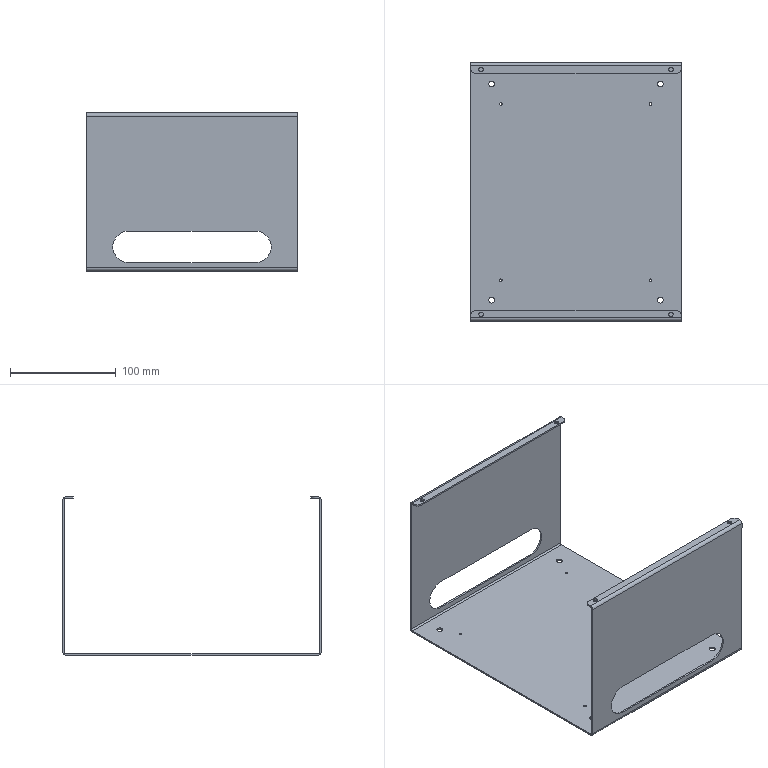Part | NX | features BREP 1 | 1 solid | 46 faces | box 200 x 245 x 150 mm | volume 153333 mm3 | cylinder 28 | plane 18 | commonest cylinder face diameters 2.5 x4 3 x4 4.2 x4 5.5 x4 6 x4 10 x4
STEP:
#1=CARTESIAN_POINT('',(-69.998,-83.5,0.));
#2=VERTEX_POINT('',#1);
#3=CARTESIAN_POINT('',(-71.248,-83.5,0.));
#4=DIRECTION('',(0.,0.,1.));
#5=DIRECTION('',(1.,0.,0.));
#6=AXIS2_PLACEMENT_3D('',#3,#4,#5);
#7=CIRCLE('',#6,1.25);
#8=EDGE_CURVE('',#2,#2,#7,.T.);
#9=ORIENTED_EDGE('',*,*,#8,.T.);
#10=EDGE_LOOP('',(#9));
#11=FACE_BOUND('',#10,.T.);
#12=CARTESIAN_POINT('',(-69.998,-83.5,-1.5));
#13=VERTEX_POINT('',#12);
#14=CARTESIAN_POINT('',(-71.248,-83.5,-1.5));
#15=DIRECTION('',(0.,0.,1.));
#16=DIRECTION('',(1.,0.,0.));
#17=AXIS2_PLACEMENT_3D('',#14,#15,#16);
#18=CIRCLE('',#17,1.25);
#19=EDGE_CURVE('',#13,#13,#18,.T.);
#20=ORIENTED_EDGE('',*,*,#19,.F.);
#21=EDGE_LOOP('',(#20));
#22=FACE_BOUND('',#21,.T.);
#23=CARTESIAN_POINT('',(-71.248,-83.5,0.));
#24=DIRECTION('',(0.,0.,1.));
#25=DIRECTION('',(1.,0.,0.));
#26=AXIS2_PLACEMENT_3D('',#23,#24,#25);
#27=CYLINDRICAL_SURFACE('',#26,1.25);
#28=ADVANCED_FACE('',(#11,#22),#27,.F.);
#29=CARTESIAN_POINT('',(72.002,-83.5,0.));
#30=VERTEX_POINT('',#29);
#31=CARTESIAN_POINT('',(70.752,-83.5,0.));
#32=DIRECTION('',(0.,0.,1.));
#33=DIRECTION('',(1.,0.,0.));
#34=AXIS2_PLACEMENT_3D('',#31,#32,#33);
#35=CIRCLE('',#34,1.25);
#36=EDGE_CURVE('',#30,#30,#35,.T.);
#37=ORIENTED_EDGE('',*,*,#36,.T.);
#38=EDGE_LOOP('',(#37));
#39=FACE_BOUND('',#38,.T.);
#40=CARTESIAN_POINT('',(72.002,-83.5,-1.5));
#41=VERTEX_POINT('',#40);
#42=CARTESIAN_POINT('',(70.752,-83.5,-1.5));
#43=DIRECTION('',(0.,0.,1.));
#44=DIRECTION('',(1.,0.,0.));
#45=AXIS2_PLACEMENT_3D('',#42,#43,#44);
#46=CIRCLE('',#45,1.25);
#47=EDGE_CURVE('',#41,#41,#46,.T.);
#48=ORIENTED_EDGE('',*,*,#47,.F.);
#49=EDGE_LOOP('',(#48));
#50=FACE_BOUND('',#49,.T.);
#51=CARTESIAN_POINT('',(70.752,-83.5,0.));
#52=DIRECTION('',(0.,0.,1.));
#53=DIRECTION('',(1.,0.,0.));
#54=AXIS2_PLACEMENT_3D('',#51,#52,#53);
#55=CYLINDRICAL_SURFACE('',#54,1.25);
#56=ADVANCED_FACE('',(#39,#50),#55,.F.);
#57=CARTESIAN_POINT('',(72.002,83.5,0.));
#58=VERTEX_POINT('',#57);
#59=CARTESIAN_POINT('',(70.752,83.5,0.));
#60=DIRECTION('',(0.,0.,1.));
#61=DIRECTION('',(1.,0.,0.));
#62=AXIS2_PLACEMENT_3D('',#59,#60,#61);
#63=CIRCLE('',#62,1.25);
#64=EDGE_CURVE('',#58,#58,#63,.T.);
#65=ORIENTED_EDGE('',*,*,#64,.T.);
#66=EDGE_LOOP('',(#65));
#67=FACE_BOUND('',#66,.T.);
#68=CARTESIAN_POINT('',(72.002,83.5,-1.5));
#69=VERTEX_POINT('',#68);
#70=CARTESIAN_POINT('',(70.752,83.5,-1.5));
#71=DIRECTION('',(0.,0.,1.));
#72=DIRECTION('',(1.,0.,0.));
#73=AXIS2_PLACEMENT_3D('',#70,#71,#72);
#74=CIRCLE('',#73,1.25);
#75=EDGE_CURVE('',#69,#69,#74,.T.);
#76=ORIENTED_EDGE('',*,*,#75,.F.);
#77=EDGE_LOOP('',(#76));
#78=FACE_BOUND('',#77,.T.);
#79=CARTESIAN_POINT('',(70.752,83.5,0.));
#80=DIRECTION('',(0.,0.,1.));
#81=DIRECTION('',(1.,0.,0.));
#82=AXIS2_PLACEMENT_3D('',#79,#80,#81);
#83=CYLINDRICAL_SURFACE('',#82,1.25);
#84=ADVANCED_FACE('',(#67,#78),#83,.F.);
#85=CARTESIAN_POINT('',(-69.998,83.5,0.));
#86=VERTEX_POINT('',#85);
#87=CARTESIAN_POINT('',(-71.248,83.5,0.));
#88=DIRECTION('',(0.,0.,1.));
#89=DIRECTION('',(1.,0.,0.));
#90=AXIS2_PLACEMENT_3D('',#87,#88,#89);
#91=CIRCLE('',#90,1.25);
#92=EDGE_CURVE('',#86,#86,#91,.T.);
#93=ORIENTED_EDGE('',*,*,#92,.T.);
#94=EDGE_LOOP('',(#93));
#95=FACE_BOUND('',#94,.T.);
#96=CARTESIAN_POINT('',(-69.998,83.5,-1.5));
#97=VERTEX_POINT('',#96);
#98=CARTESIAN_POINT('',(-71.248,83.5,-1.5));
#99=DIRECTION('',(0.,0.,1.));
#100=DIRECTION('',(1.,0.,0.));
#101=AXIS2_PLACEMENT_3D('',#98,#99,#100);
#102=CIRCLE('',#101,1.25);
#103=EDGE_CURVE('',#97,#97,#102,.T.);
#104=ORIENTED_EDGE('',*,*,#103,.F.);
#105=EDGE_LOOP('',(#104));
#106=FACE_BOUND('',#105,.T.);
#107=CARTESIAN_POINT('',(-71.248,83.5,0.));
#108=DIRECTION('',(0.,0.,1.));
#109=DIRECTION('',(1.,0.,0.));
#110=AXIS2_PLACEMENT_3D('',#107,#108,#109);
#111=CYLINDRICAL_SURFACE('',#110,1.25);
#112=ADVANCED_FACE('',(#95,#106),#111,.F.);
#113=CARTESIAN_POINT('',(92.1,116.,148.5));
#114=VERTEX_POINT('',#113);
#115=CARTESIAN_POINT('',(90.,116.,148.5));
#116=DIRECTION('',(0.,0.,1.));
#117=DIRECTION('',(1.,0.,0.));
#118=AXIS2_PLACEMENT_3D('',#115,#116,#117);
#119=CIRCLE('',#118,2.1);
#120=EDGE_CURVE('',#114,#114,#119,.T.);
#121=ORIENTED_EDGE('',*,*,#120,.T.);
#122=EDGE_LOOP('',(#121));
#123=FACE_BOUND('',#122,.T.);
#124=CARTESIAN_POINT('',(90.,113.9,147.));
#125=VERTEX_POINT('',#124);
#126=CARTESIAN_POINT('',(90.,116.,147.));
#127=DIRECTION('',(0.,0.,1.));
#128=DIRECTION('',(0.,-1.,0.));
#129=AXIS2_PLACEMENT_3D('',#126,#127,#128);
#130=CIRCLE('',#129,2.1);
#131=EDGE_CURVE('',#125,#125,#130,.T.);
#132=ORIENTED_EDGE('',*,*,#131,.F.);
#133=EDGE_LOOP('',(#132));
#134=FACE_BOUND('',#133,.T.);
#135=CARTESIAN_POINT('',(90.,116.,148.5));
#136=DIRECTION('',(0.,0.,1.));
#137=DIRECTION('',(1.,0.,0.));
#138=AXIS2_PLACEMENT_3D('',#135,#136,#137);
#139=CYLINDRICAL_SURFACE('',#138,2.1);
#140=ADVANCED_FACE('',(#123,#134),#139,.F.);
#141=CARTESIAN_POINT('',(-87.9,116.,148.5));
#142=VERTEX_POINT('',#141);
#143=CARTESIAN_POINT('',(-90.,116.,148.5));
#144=DIRECTION('',(0.,0.,1.));
#145=DIRECTION('',(1.,0.,0.));
#146=AXIS2_PLACEMENT_3D('',#143,#144,#145);
#147=CIRCLE('',#146,2.1);
#148=EDGE_CURVE('',#142,#142,#147,.T.);
#149=ORIENTED_EDGE('',*,*,#148,.T.);
#150=EDGE_LOOP('',(#149));
#151=FACE_BOUND('',#150,.T.);
#152=CARTESIAN_POINT('',(-90.,113.9,147.));
#153=VERTEX_POINT('',#152);
#154=CARTESIAN_POINT('',(-90.,116.,147.));
#155=DIRECTION('',(0.,0.,1.));
#156=DIRECTION('',(0.,-1.,0.));
#157=AXIS2_PLACEMENT_3D('',#154,#155,#156);
#158=CIRCLE('',#157,2.1);
#159=EDGE_CURVE('',#153,#153,#158,.T.);
#160=ORIENTED_EDGE('',*,*,#159,.F.);
#161=EDGE_LOOP('',(#160));
#162=FACE_BOUND('',#161,.T.);
#163=CARTESIAN_POINT('',(-90.,116.,148.5));
#164=DIRECTION('',(0.,0.,1.));
#165=DIRECTION('',(1.,0.,0.));
#166=AXIS2_PLACEMENT_3D('',#163,#164,#165);
#167=CYLINDRICAL_SURFACE('',#166,2.1);
#168=ADVANCED_FACE('',(#151,#162),#167,.F.);
#169=CARTESIAN_POINT('',(-87.9,-116.,148.5));
#170=VERTEX_POINT('',#169);
#171=CARTESIAN_POINT('',(-90.,-116.,148.5));
#172=DIRECTION('',(0.,0.,1.));
#173=DIRECTION('',(1.,0.,0.));
#174=AXIS2_PLACEMENT_3D('',#171,#172,#173);
#175=CIRCLE('',#174,2.1);
#176=EDGE_CURVE('',#170,#170,#175,.T.);
#177=ORIENTED_EDGE('',*,*,#176,.T.);
#178=EDGE_LOOP('',(#177));
#179=FACE_BOUND('',#178,.T.);
#180=CARTESIAN_POINT('',(-90.,-113.9,147.));
#181=VERTEX_POINT('',#180);
#182=CARTESIAN_POINT('',(-90.,-116.,147.));
#183=DIRECTION('',(0.,0.,-1.));
#184=DIRECTION('',(0.,1.,0.));
#185=AXIS2_PLACEMENT_3D('',#182,#183,#184);
#186=CIRCLE('',#185,2.1);
#187=EDGE_CURVE('',#181,#181,#186,.T.);
#188=ORIENTED_EDGE('',*,*,#187,.T.);
#189=EDGE_LOOP('',(#188));
#190=FACE_BOUND('',#189,.T.);
#191=CARTESIAN_POINT('',(-90.,-116.,148.5));
#192=DIRECTION('',(0.,0.,1.));
#193=DIRECTION('',(1.,0.,0.));
#194=AXIS2_PLACEMENT_3D('',#191,#192,#193);
#195=CYLINDRICAL_SURFACE('',#194,2.1);
#196=ADVANCED_FACE('',(#179,#190),#195,.F.);
#197=CARTESIAN_POINT('',(92.1,-116.,148.5));
#198=VERTEX_POINT('',#197);
#199=CARTESIAN_POINT('',(90.,-116.,148.5));
#200=DIRECTION('',(0.,0.,1.));
#201=DIRECTION('',(1.,0.,0.));
#202=AXIS2_PLACEMENT_3D('',#199,#200,#201);
#203=CIRCLE('',#202,2.1);
#204=EDGE_CURVE('',#198,#198,#203,.T.);
#205=ORIENTED_EDGE('',*,*,#204,.T.);
#206=EDGE_LOOP('',(#205));
#207=FACE_BOUND('',#206,.T.);
#208=CARTESIAN_POINT('',(90.,-113.9,147.));
#209=VERTEX_POINT('',#208);
#210=CARTESIAN_POINT('',(90.,-116.,147.));
#211=DIRECTION('',(0.,0.,-1.));
#212=DIRECTION('',(0.,1.,0.));
#213=AXIS2_PLACEMENT_3D('',#210,#211,#212);
#214=CIRCLE('',#213,2.1);
#215=EDGE_CURVE('',#209,#209,#214,.T.);
#216=ORIENTED_EDGE('',*,*,#215,.T.);
#217=EDGE_LOOP('',(#216));
#218=FACE_BOUND('',#217,.T.);
#219=CARTESIAN_POINT('',(90.,-116.,148.5));
#220=DIRECTION('',(0.,0.,1.));
#221=DIRECTION('',(1.,0.,0.));
#222=AXIS2_PLACEMENT_3D('',#219,#220,#221);
#223=CYLINDRICAL_SURFACE('',#222,2.1);
#224=ADVANCED_FACE('',(#207,#218),#223,.F.);
#225=CARTESIAN_POINT('',(-82.75,-102.5,0.));
#226=VERTEX_POINT('',#225);
#227=CARTESIAN_POINT('',(-80.,-102.5,0.));
#228=DIRECTION('',(0.,0.,1.));
#229=DIRECTION('',(-1.,0.,0.));
#230=AXIS2_PLACEMENT_3D('',#227,#228,#229);
#231=CIRCLE('',#230,2.75);
#232=EDGE_CURVE('',#226,#226,#231,.T.);
#233=ORIENTED_EDGE('',*,*,#232,.T.);
#234=EDGE_LOOP('',(#233));
#235=FACE_BOUND('',#234,.T.);
#236=CARTESIAN_POINT('',(-82.75,-102.5,-1.5));
#237=VERTEX_POINT('',#236);
#238=CARTESIAN_POINT('',(-80.,-102.5,-1.5));
#239=DIRECTION('',(0.,0.,-1.));
#240=DIRECTION('',(-1.,0.,0.));
#241=AXIS2_PLACEMENT_3D('',#238,#239,#240);
#242=CIRCLE('',#241,2.75);
#243=EDGE_CURVE('',#237,#237,#242,.T.);
#244=ORIENTED_EDGE('',*,*,#243,.T.);
#245=EDGE_LOOP('',(#244));
#246=FACE_BOUND('',#245,.T.);
#247=CARTESIAN_POINT('',(-80.,-102.5,-10.));
#248=DIRECTION('',(0.,0.,1.));
#249=DIRECTION('',(1.,0.,0.));
#250=AXIS2_PLACEMENT_3D('',#247,#248,#249);
#251=CYLINDRICAL_SURFACE('',#250,2.75);
#252=ADVANCED_FACE('',(#235,#246),#251,.F.);
#253=CARTESIAN_POINT('',(82.75,-102.5,0.));
#254=VERTEX_POINT('',#253);
#255=CARTESIAN_POINT('',(80.,-102.5,0.));
#256=DIRECTION('',(0.,0.,1.));
#257=DIRECTION('',(1.,0.,0.));
#258=AXIS2_PLACEMENT_3D('',#255,#256,#257);
#259=CIRCLE('',#258,2.75);
#260=EDGE_CURVE('',#254,#254,#259,.T.);
#261=ORIENTED_EDGE('',*,*,#260,.T.);
#262=EDGE_LOOP('',(#261));
#263=FACE_BOUND('',#262,.T.);
#264=CARTESIAN_POINT('',(77.25,-102.5,-1.5));
#265=VERTEX_POINT('',#264);
#266=CARTESIAN_POINT('',(80.,-102.5,-1.5));
#267=DIRECTION('',(0.,0.,-1.));
#268=DIRECTION('',(-1.,0.,0.));
#269=AXIS2_PLACEMENT_3D('',#266,#267,#268);
#270=CIRCLE('',#269,2.75);
#271=EDGE_CURVE('',#265,#265,#270,.T.);
#272=ORIENTED_EDGE('',*,*,#271,.T.);
#273=EDGE_LOOP('',(#272));
#274=FACE_BOUND('',#273,.T.);
#275=CARTESIAN_POINT('',(80.,-102.5,-10.));
#276=DIRECTION('',(0.,0.,1.));
#277=DIRECTION('',(1.,0.,0.));
#278=AXIS2_PLACEMENT_3D('',#275,#276,#277);
#279=CYLINDRICAL_SURFACE('',#278,2.75);
#280=ADVANCED_FACE('',(#263,#274),#279,.F.);
#281=CARTESIAN_POINT('',(77.25,102.5,0.));
#282=VERTEX_POINT('',#281);
#283=CARTESIAN_POINT('',(80.,102.5,0.));
#284=DIRECTION('',(0.,0.,1.));
#285=DIRECTION('',(-1.,0.,0.));
#286=AXIS2_PLACEMENT_3D('',#283,#284,#285);
#287=CIRCLE('',#286,2.75);
#288=EDGE_CURVE('',#282,#282,#287,.T.);
#289=ORIENTED_EDGE('',*,*,#288,.T.);
#290=EDGE_LOOP('',(#289));
#291=FACE_BOUND('',#290,.T.);
#292=CARTESIAN_POINT('',(77.25,102.5,-1.5));
#293=VERTEX_POINT('',#292);
#294=CARTESIAN_POINT('',(80.,102.5,-1.5));
#295=DIRECTION('',(0.,0.,-1.));
#296=DIRECTION('',(-1.,0.,0.));
#297=AXIS2_PLACEMENT_3D('',#294,#295,#296);
#298=CIRCLE('',#297,2.75);
#299=EDGE_CURVE('',#293,#293,#298,.T.);
#300=ORIENTED_EDGE('',*,*,#299,.T.);
#301=EDGE_LOOP('',(#300));
#302=FACE_BOUND('',#301,.T.);
#303=CARTESIAN_POINT('',(80.,102.5,-10.));
#304=DIRECTION('',(0.,0.,1.));
#305=DIRECTION('',(1.,0.,0.));
#306=AXIS2_PLACEMENT_3D('',#303,#304,#305);
#307=CYLINDRICAL_SURFACE('',#306,2.75);
#308=ADVANCED_FACE('',(#291,#302),#307,.F.);
#309=CARTESIAN_POINT('',(-77.25,102.5,0.));
#310=VERTEX_POINT('',#309);
#311=CARTESIAN_POINT('',(-80.,102.5,0.));
#312=DIRECTION('',(0.,0.,1.));
#313=DIRECTION('',(1.,0.,0.));
#314=AXIS2_PLACEMENT_3D('',#311,#312,#313);
#315=CIRCLE('',#314,2.75);
#316=EDGE_CURVE('',#310,#310,#315,.T.);
#317=ORIENTED_EDGE('',*,*,#316,.T.);
#318=EDGE_LOOP('',(#317));
#319=FACE_BOUND('',#318,.T.);
#320=CARTESIAN_POINT('',(-82.75,102.5,-1.5));
#321=VERTEX_POINT('',#320);
#322=CARTESIAN_POINT('',(-80.,102.5,-1.5));
#323=DIRECTION('',(0.,0.,-1.));
#324=DIRECTION('',(-1.,0.,0.));
#325=AXIS2_PLACEMENT_3D('',#322,#323,#324);
#326=CIRCLE('',#325,2.75);
#327=EDGE_CURVE('',#321,#321,#326,.T.);
#328=ORIENTED_EDGE('',*,*,#327,.T.);
#329=EDGE_LOOP('',(#328));
#330=FACE_BOUND('',#329,.T.);
#331=CARTESIAN_POINT('',(-80.,102.5,-10.));
#332=DIRECTION('',(0.,0.,1.));
#333=DIRECTION('',(1.,0.,0.));
#334=AXIS2_PLACEMENT_3D('',#331,#332,#333);
#335=CYLINDRICAL_SURFACE('',#334,2.75);
#336=ADVANCED_FACE('',(#319,#330),#335,.F.);
#337=ORIENTED_EDGE('',*,*,#19,.T.);
#338=EDGE_LOOP('',(#337));
#339=FACE_BOUND('',#338,.T.);
#340=ORIENTED_EDGE('',*,*,#47,.T.);
#341=EDGE_LOOP('',(#340));
#342=FACE_BOUND('',#341,.T.);
#343=ORIENTED_EDGE('',*,*,#75,.T.);
#344=EDGE_LOOP('',(#343));
#345=FACE_BOUND('',#344,.T.);
#346=CARTESIAN_POINT('',(-100.,119.5,-1.5));
#347=VERTEX_POINT('',#346);
#348=CARTESIAN_POINT('',(-100.,-119.5,-1.5));
#349=VERTEX_POINT('',#348);
#350=CARTESIAN_POINT('',(-100.,-122.5,-1.5));
#351=DIRECTION('',(0.,-1.,0.));
#352=VECTOR('',#351,1000.);
#353=LINE('',#350,#352);
#354=EDGE_CURVE('',#347,#349,#353,.T.);
#355=ORIENTED_EDGE('',*,*,#354,.F.);
#356=CARTESIAN_POINT('',(100.,119.5,-1.5));
#357=VERTEX_POINT('',#356);
#358=CARTESIAN_POINT('',(-100.,119.5,-1.5));
#359=DIRECTION('',(1.,0.,0.));
#360=VECTOR('',#359,1000.);
#361=LINE('',#358,#360);
#362=EDGE_CURVE('',#347,#357,#361,.T.);
#363=ORIENTED_EDGE('',*,*,#362,.T.);
#364=CARTESIAN_POINT('',(100.,-119.5,-1.5));
#365=VERTEX_POINT('',#364);
#366=CARTESIAN_POINT('',(100.,-122.5,-1.5));
#367=DIRECTION('',(0.,1.,0.));
#368=VECTOR('',#367,1000.);
#369=LINE('',#366,#368);
#370=EDGE_CURVE('',#365,#357,#369,.T.);
#371=ORIENTED_EDGE('',*,*,#370,.F.);
#372=CARTESIAN_POINT('',(100.,-119.5,-1.5));
#373=DIRECTION('',(-1.,0.,0.));
#374=VECTOR('',#373,1000.);
#375=LINE('',#372,#374);
#376=EDGE_CURVE('',#365,#349,#375,.T.);
#377=ORIENTED_EDGE('',*,*,#376,.T.);
#378=EDGE_LOOP('',(#355,#363,#371,#377));
#379=FACE_BOUND('',#378,.T.);
#380=ORIENTED_EDGE('',*,*,#327,.F.);
#381=EDGE_LOOP('',(#380));
#382=FACE_BOUND('',#381,.T.);
#383=ORIENTED_EDGE('',*,*,#299,.F.);
#384=EDGE_LOOP('',(#383));
#385=FACE_BOUND('',#384,.T.);
#386=ORIENTED_EDGE('',*,*,#271,.F.);
#387=EDGE_LOOP('',(#386));
#388=FACE_BOUND('',#387,.T.);
#389=ORIENTED_EDGE('',*,*,#243,.F.);
#390=EDGE_LOOP('',(#389));
#391=FACE_BOUND('',#390,.T.);
#392=ORIENTED_EDGE('',*,*,#103,.T.);
#393=EDGE_LOOP('',(#392));
#394=FACE_BOUND('',#393,.T.);
#395=CARTESIAN_POINT('',(0.,0.,-1.5));
#396=DIRECTION('',(0.,0.,-1.));
#397=DIRECTION('',(-1.,0.,0.));
#398=AXIS2_PLACEMENT_3D('',#395,#396,#397);
#399=PLANE('',#398);
#400=ADVANCED_FACE('',(#339,#342,#345,#379,#382,#385,#388,#391,#394),#399,.T.);
#401=CARTESIAN_POINT('',(100.,-122.5,145.5));
#402=VERTEX_POINT('',#401);
#403=CARTESIAN_POINT('',(-100.,-122.5,145.5));
#404=VERTEX_POINT('',#403);
#405=CARTESIAN_POINT('',(100.,-122.5,145.5));
#406=DIRECTION('',(-1.,0.,0.));
#407=VECTOR('',#406,1000.);
#408=LINE('',#405,#407);
#409=EDGE_CURVE('',#402,#404,#408,.T.);
#410=ORIENTED_EDGE('',*,*,#409,.T.);
#411=CARTESIAN_POINT('',(-100.,-122.5,1.5));
#412=VERTEX_POINT('',#411);
#413=CARTESIAN_POINT('',(-100.,-122.5,0.));
#414=DIRECTION('',(0.,0.,-1.));
#415=VECTOR('',#414,1000.);
#416=LINE('',#413,#415);
#417=EDGE_CURVE('',#404,#412,#416,.T.);
#418=ORIENTED_EDGE('',*,*,#417,.T.);
#419=CARTESIAN_POINT('',(100.,-122.5,1.5));
#420=VERTEX_POINT('',#419);
#421=CARTESIAN_POINT('',(-100.,-122.5,1.5));
#422=DIRECTION('',(-1.,0.,0.));
#423=VECTOR('',#422,1000.);
#424=LINE('',#421,#423);
#425=EDGE_CURVE('',#420,#412,#424,.T.);
#426=ORIENTED_EDGE('',*,*,#425,.F.);
#427=CARTESIAN_POINT('',(100.,-122.5,0.));
#428=DIRECTION('',(0.,0.,1.));
#429=VECTOR('',#428,1000.);
#430=LINE('',#427,#429);
#431=EDGE_CURVE('',#420,#402,#430,.T.);
#432=ORIENTED_EDGE('',*,*,#431,.T.);
#433=EDGE_LOOP('',(#410,#418,#426,#432));
#434=FACE_BOUND('',#433,.T.);
#435=CARTESIAN_POINT('',(-60.,-122.5,36.5));
#436=VERTEX_POINT('',#435);
#437=CARTESIAN_POINT('',(60.,-122.5,36.5));
#438=VERTEX_POINT('',#437);
#439=CARTESIAN_POINT('',(75.,-122.5,36.5));
#440=DIRECTION('',(1.,0.,0.));
#441=VECTOR('',#440,1000.);
#442=LINE('',#439,#441);
#443=EDGE_CURVE('',#436,#438,#442,.T.);
#444=ORIENTED_EDGE('',*,*,#443,.T.);
#445=CARTESIAN_POINT('',(60.,-122.5,6.5));
#446=VERTEX_POINT('',#445);
#447=CARTESIAN_POINT('',(60.,-122.5,21.5));
#448=DIRECTION('',(0.,1.,0.));
#449=DIRECTION('',(0.,0.,1.));
#450=AXIS2_PLACEMENT_3D('',#447,#448,#449);
#451=CIRCLE('',#450,15.);
#452=EDGE_CURVE('',#438,#446,#451,.T.);
#453=ORIENTED_EDGE('',*,*,#452,.T.);
#454=CARTESIAN_POINT('',(-60.,-122.5,6.5));
#455=VERTEX_POINT('',#454);
#456=CARTESIAN_POINT('',(75.,-122.5,6.5));
#457=DIRECTION('',(-1.,0.,0.));
#458=VECTOR('',#457,1000.);
#459=LINE('',#456,#458);
#460=EDGE_CURVE('',#446,#455,#459,.T.);
#461=ORIENTED_EDGE('',*,*,#460,.T.);
#462=CARTESIAN_POINT('',(-60.,-122.5,21.5));
#463=DIRECTION('',(0.,1.,0.));
#464=DIRECTION('',(0.,0.,1.));
#465=AXIS2_PLACEMENT_3D('',#462,#463,#464);
#466=CIRCLE('',#465,15.);
#467=EDGE_CURVE('',#455,#436,#466,.T.);
#468=ORIENTED_EDGE('',*,*,#467,.T.);
#469=EDGE_LOOP('',(#444,#453,#461,#468));
#470=FACE_BOUND('',#469,.T.);
#471=CARTESIAN_POINT('',(0.,-122.5,0.));
#472=DIRECTION('',(0.,1.,0.));
#473=DIRECTION('',(0.,0.,1.));
#474=AXIS2_PLACEMENT_3D('',#471,#472,#473);
#475=PLANE('',#474);
#476=ADVANCED_FACE('',(#434,#470),#475,.F.);
#477=CARTESIAN_POINT('',(-100.,-121.,145.5));
#478=VERTEX_POINT('',#477);
#479=CARTESIAN_POINT('',(-100.,-121.,1.5));
#480=VERTEX_POINT('',#479);
#481=CARTESIAN_POINT('',(-100.,-121.,0.));
#482=DIRECTION('',(0.,0.,-1.));
#483=VECTOR('',#482,1000.);
#484=LINE('',#481,#483);
#485=EDGE_CURVE('',#478,#480,#484,.T.);
#486=ORIENTED_EDGE('',*,*,#485,.F.);
#487=CARTESIAN_POINT('',(100.,-121.,145.5));
#488=VERTEX_POINT('',#487);
#489=CARTESIAN_POINT('',(100.,-121.,145.5));
#490=DIRECTION('',(-1.,0.,0.));
#491=VECTOR('',#490,1000.);
#492=LINE('',#489,#491);
#493=EDGE_CURVE('',#488,#478,#492,.T.);
#494=ORIENTED_EDGE('',*,*,#493,.F.);
#495=CARTESIAN_POINT('',(100.,-121.,1.5));
#496=VERTEX_POINT('',#495);
#497=CARTESIAN_POINT('',(100.,-121.,148.5));
#498=DIRECTION('',(0.,0.,1.));
#499=VECTOR('',#498,1000.);
#500=LINE('',#497,#499);
#501=EDGE_CURVE('',#496,#488,#500,.T.);
#502=ORIENTED_EDGE('',*,*,#501,.F.);
#503=CARTESIAN_POINT('',(-100.,-121.,1.5));
#504=DIRECTION('',(1.,0.,0.));
#505=VECTOR('',#504,1000.);
#506=LINE('',#503,#505);
#507=EDGE_CURVE('',#480,#496,#506,.T.);
#508=ORIENTED_EDGE('',*,*,#507,.F.);
#509=EDGE_LOOP('',(#486,#494,#502,#508));
#510=FACE_BOUND('',#509,.T.);
#511=CARTESIAN_POINT('',(60.,-121.,36.5));
#512=VERTEX_POINT('',#511);
#513=CARTESIAN_POINT('',(-60.,-121.,36.5));
#514=VERTEX_POINT('',#513);
#515=CARTESIAN_POINT('',(0.,-121.,36.5));
#516=DIRECTION('',(-1.,0.,0.));
#517=VECTOR('',#516,1000.);
#518=LINE('',#515,#517);
#519=EDGE_CURVE('',#512,#514,#518,.T.);
#520=ORIENTED_EDGE('',*,*,#519,.T.);
#521=CARTESIAN_POINT('',(-60.,-121.,6.5));
#522=VERTEX_POINT('',#521);
#523=CARTESIAN_POINT('',(-60.,-121.,21.5));
#524=DIRECTION('',(0.,-1.,0.));
#525=DIRECTION('',(0.,0.,1.));
#526=AXIS2_PLACEMENT_3D('',#523,#524,#525);
#527=CIRCLE('',#526,15.);
#528=EDGE_CURVE('',#514,#522,#527,.T.);
#529=ORIENTED_EDGE('',*,*,#528,.T.);
#530=CARTESIAN_POINT('',(60.,-121.,6.5));
#531=VERTEX_POINT('',#530);
#532=CARTESIAN_POINT('',(0.,-121.,6.5));
#533=DIRECTION('',(1.,0.,0.));
#534=VECTOR('',#533,1000.);
#535=LINE('',#532,#534);
#536=EDGE_CURVE('',#522,#531,#535,.T.);
#537=ORIENTED_EDGE('',*,*,#536,.T.);
#538=CARTESIAN_POINT('',(60.,-121.,21.5));
#539=DIRECTION('',(0.,-1.,0.));
#540=DIRECTION('',(0.,0.,1.));
#541=AXIS2_PLACEMENT_3D('',#538,#539,#540);
#542=CIRCLE('',#541,15.);
#543=EDGE_CURVE('',#531,#512,#542,.T.);
#544=ORIENTED_EDGE('',*,*,#543,.T.);
#545=EDGE_LOOP('',(#520,#529,#537,#544));
#546=FACE_BOUND('',#545,.T.);
#547=CARTESIAN_POINT('',(0.,-121.,0.));
#548=DIRECTION('',(0.,1.,0.));
#549=DIRECTION('',(0.,0.,1.));
#550=AXIS2_PLACEMENT_3D('',#547,#548,#549);
#551=PLANE('',#550);
#552=ADVANCED_FACE('',(#510,#546),#551,.T.);
#553=ORIENTED_EDGE('',*,*,#417,.F.);
#554=CARTESIAN_POINT('',(-100.,-119.5,148.5));
#555=VERTEX_POINT('',#554);
#556=CARTESIAN_POINT('',(-100.,-119.5,145.5));
#557=DIRECTION('',(-1.,0.,0.));
#558=DIRECTION('',(0.,0.,-1.));
#559=AXIS2_PLACEMENT_3D('',#556,#557,#558);
#560=CIRCLE('',#559,3.);
#561=EDGE_CURVE('',#404,#555,#560,.T.);
#562=ORIENTED_EDGE('',*,*,#561,.T.);
#563=CARTESIAN_POINT('',(-100.,-117.5,148.5));
#564=VERTEX_POINT('',#563);
#565=CARTESIAN_POINT('',(-100.,-121.,148.5));
#566=DIRECTION('',(0.,1.,0.));
#567=VECTOR('',#566,1000.);
#568=LINE('',#565,#567);
#569=EDGE_CURVE('',#555,#564,#568,.T.);
#570=ORIENTED_EDGE('',*,*,#569,.T.);
#571=CARTESIAN_POINT('',(-100.,-117.5,147.));
#572=VERTEX_POINT('',#571);
#573=CARTESIAN_POINT('',(-100.,-117.5,148.5));
#574=DIRECTION('',(0.,0.,-1.));
#575=VECTOR('',#574,1000.);
#576=LINE('',#573,#575);
#577=EDGE_CURVE('',#564,#572,#576,.T.);
#578=ORIENTED_EDGE('',*,*,#577,.T.);
#579=CARTESIAN_POINT('',(-100.,-119.5,147.));
#580=VERTEX_POINT('',#579);
#581=CARTESIAN_POINT('',(-100.,0.,147.));
#582=DIRECTION('',(0.,1.,0.));
#583=VECTOR('',#582,1000.);
#584=LINE('',#581,#583);
#585=EDGE_CURVE('',#580,#572,#584,.T.);
#586=ORIENTED_EDGE('',*,*,#585,.F.);
#587=CARTESIAN_POINT('',(-100.,-119.5,145.5));
#588=DIRECTION('',(-1.,0.,0.));
#589=DIRECTION('',(0.,0.,-1.));
#590=AXIS2_PLACEMENT_3D('',#587,#588,#589);
#591=CIRCLE('',#590,1.5);
#592=EDGE_CURVE('',#478,#580,#591,.T.);
#593=ORIENTED_EDGE('',*,*,#592,.F.);
#594=ORIENTED_EDGE('',*,*,#485,.T.);
#595=CARTESIAN_POINT('',(-100.,-119.5,0.));
#596=VERTEX_POINT('',#595);
#597=CARTESIAN_POINT('',(-100.,-119.5,1.5));
#598=DIRECTION('',(-1.,0.,0.));
#599=DIRECTION('',(0.,0.,-1.));
#600=AXIS2_PLACEMENT_3D('',#597,#598,#599);
#601=CIRCLE('',#600,1.5);
#602=EDGE_CURVE('',#596,#480,#601,.T.);
#603=ORIENTED_EDGE('',*,*,#602,.F.);
#604=CARTESIAN_POINT('',(-100.,119.5,0.));
#605=VERTEX_POINT('',#604);
#606=CARTESIAN_POINT('',(-100.,-122.5,0.));
#607=DIRECTION('',(0.,-1.,0.));
#608=VECTOR('',#607,1000.);
#609=LINE('',#606,#608);
#610=EDGE_CURVE('',#605,#596,#609,.T.);
#611=ORIENTED_EDGE('',*,*,#610,.F.);
#612=CARTESIAN_POINT('',(-100.,121.,1.5));
#613=VERTEX_POINT('',#612);
#614=CARTESIAN_POINT('',(-100.,119.5,1.5));
#615=DIRECTION('',(-1.,0.,0.));
#616=DIRECTION('',(0.,0.,1.));
#617=AXIS2_PLACEMENT_3D('',#614,#615,#616);
#618=CIRCLE('',#617,1.5);
#619=EDGE_CURVE('',#613,#605,#618,.T.);
#620=ORIENTED_EDGE('',*,*,#619,.F.);
#621=CARTESIAN_POINT('',(-100.,121.,145.5));
#622=VERTEX_POINT('',#621);
#623=CARTESIAN_POINT('',(-100.,121.,148.5));
#624=DIRECTION('',(0.,0.,1.));
#625=VECTOR('',#624,1000.);
#626=LINE('',#623,#625);
#627=EDGE_CURVE('',#613,#622,#626,.T.);
#628=ORIENTED_EDGE('',*,*,#627,.T.);
#629=CARTESIAN_POINT('',(-100.,119.5,147.));
#630=VERTEX_POINT('',#629);
#631=CARTESIAN_POINT('',(-100.,119.5,145.5));
#632=DIRECTION('',(-1.,0.,0.));
#633=DIRECTION('',(0.,0.,1.));
#634=AXIS2_PLACEMENT_3D('',#631,#632,#633);
#635=CIRCLE('',#634,1.5);
#636=EDGE_CURVE('',#630,#622,#635,.T.);
#637=ORIENTED_EDGE('',*,*,#636,.F.);
#638=CARTESIAN_POINT('',(-100.,117.5,147.));
#639=VERTEX_POINT('',#638);
#640=CARTESIAN_POINT('',(-100.,0.,147.));
#641=DIRECTION('',(0.,1.,0.));
#642=VECTOR('',#641,1000.);
#643=LINE('',#640,#642);
#644=EDGE_CURVE('',#639,#630,#643,.T.);
#645=ORIENTED_EDGE('',*,*,#644,.F.);
#646=CARTESIAN_POINT('',(-100.,117.5,148.5));
#647=VERTEX_POINT('',#646);
#648=CARTESIAN_POINT('',(-100.,117.5,148.5));
#649=DIRECTION('',(0.,0.,1.));
#650=VECTOR('',#649,1000.);
#651=LINE('',#648,#650);
#652=EDGE_CURVE('',#639,#647,#651,.T.);
#653=ORIENTED_EDGE('',*,*,#652,.T.);
#654=CARTESIAN_POINT('',(-100.,119.5,148.5));
#655=VERTEX_POINT('',#654);
#656=CARTESIAN_POINT('',(-100.,121.,148.5));
#657=DIRECTION('',(0.,1.,0.));
#658=VECTOR('',#657,1000.);
#659=LINE('',#656,#658);
#660=EDGE_CURVE('',#647,#655,#659,.T.);
#661=ORIENTED_EDGE('',*,*,#660,.T.);
#662=CARTESIAN_POINT('',(-100.,122.5,145.5));
#663=VERTEX_POINT('',#662);
#664=CARTESIAN_POINT('',(-100.,119.5,145.5));
#665=DIRECTION('',(-1.,0.,0.));
#666=DIRECTION('',(0.,0.,1.));
#667=AXIS2_PLACEMENT_3D('',#664,#665,#666);
#668=CIRCLE('',#667,3.);
#669=EDGE_CURVE('',#655,#663,#668,.T.);
#670=ORIENTED_EDGE('',*,*,#669,.T.);
#671=CARTESIAN_POINT('',(-100.,122.5,1.5));
#672=VERTEX_POINT('',#671);
#673=CARTESIAN_POINT('',(-100.,122.5,0.));
#674=DIRECTION('',(0.,0.,1.));
#675=VECTOR('',#674,1000.);
#676=LINE('',#673,#675);
#677=EDGE_CURVE('',#672,#663,#676,.T.);
#678=ORIENTED_EDGE('',*,*,#677,.F.);
#679=CARTESIAN_POINT('',(-100.,119.5,1.5));
#680=DIRECTION('',(-1.,0.,0.));
#681=DIRECTION('',(0.,0.,1.));
#682=AXIS2_PLACEMENT_3D('',#679,#680,#681);
#683=CIRCLE('',#682,3.);
#684=EDGE_CURVE('',#672,#347,#683,.T.);
#685=ORIENTED_EDGE('',*,*,#684,.T.);
#686=ORIENTED_EDGE('',*,*,#354,.T.);
#687=CARTESIAN_POINT('',(-100.,-119.5,1.5));
#688=DIRECTION('',(-1.,0.,0.));
#689=DIRECTION('',(0.,0.,-1.));
#690=AXIS2_PLACEMENT_3D('',#687,#688,#689);
#691=CIRCLE('',#690,3.);
#692=EDGE_CURVE('',#349,#412,#691,.T.);
#693=ORIENTED_EDGE('',*,*,#692,.T.);
#694=EDGE_LOOP('',(#553,#562,#570,#578,#586,#593,#594,#603,#611,#620,#628,#637,#645,#653,#661,#670,#678,#685,#686,#693));
#695=FACE_BOUND('',#694,.T.);
#696=CARTESIAN_POINT('',(-100.,-122.5,0.));
#697=DIRECTION('',(1.,0.,0.));
#698=DIRECTION('',(0.,0.,-1.));
#699=AXIS2_PLACEMENT_3D('',#696,#697,#698);
#700=PLANE('',#699);
#701=ADVANCED_FACE('',(#695),#700,.F.);
#702=ORIENTED_EDGE('',*,*,#501,.T.);
#703=CARTESIAN_POINT('',(100.,-119.5,147.));
#704=VERTEX_POINT('',#703);
#705=CARTESIAN_POINT('',(100.,-119.5,145.5));
#706=DIRECTION('',(1.,0.,0.));
#707=DIRECTION('',(0.,0.,-1.));
#708=AXIS2_PLACEMENT_3D('',#705,#706,#707);
#709=CIRCLE('',#708,1.5);
#710=EDGE_CURVE('',#704,#488,#709,.T.);
#711=ORIENTED_EDGE('',*,*,#710,.F.);
#712=CARTESIAN_POINT('',(100.,-117.5,147.));
#713=VERTEX_POINT('',#712);
#714=CARTESIAN_POINT('',(100.,0.,147.));
#715=DIRECTION('',(0.,-1.,0.));
#716=VECTOR('',#715,1000.);
#717=LINE('',#714,#716);
#718=EDGE_CURVE('',#713,#704,#717,.T.);
#719=ORIENTED_EDGE('',*,*,#718,.F.);
#720=CARTESIAN_POINT('',(100.,-117.5,148.5));
#721=VERTEX_POINT('',#720);
#722=CARTESIAN_POINT('',(100.,-117.5,148.5));
#723=DIRECTION('',(0.,0.,1.));
#724=VECTOR('',#723,1000.);
#725=LINE('',#722,#724);
#726=EDGE_CURVE('',#713,#721,#725,.T.);
#727=ORIENTED_EDGE('',*,*,#726,.T.);
#728=CARTESIAN_POINT('',(100.,-119.5,148.5));
#729=VERTEX_POINT('',#728);
#730=CARTESIAN_POINT('',(100.,-112.5,148.5));
#731=DIRECTION('',(0.,-1.,0.));
#732=VECTOR('',#731,1000.);
#733=LINE('',#730,#732);
#734=EDGE_CURVE('',#721,#729,#733,.T.);
#735=ORIENTED_EDGE('',*,*,#734,.T.);
#736=CARTESIAN_POINT('',(100.,-119.5,145.5));
#737=DIRECTION('',(1.,0.,0.));
#738=DIRECTION('',(0.,0.,-1.));
#739=AXIS2_PLACEMENT_3D('',#736,#737,#738);
#740=CIRCLE('',#739,3.);
#741=EDGE_CURVE('',#729,#402,#740,.T.);
#742=ORIENTED_EDGE('',*,*,#741,.T.);
#743=ORIENTED_EDGE('',*,*,#431,.F.);
#744=CARTESIAN_POINT('',(100.,-119.5,1.5));
#745=DIRECTION('',(1.,0.,0.));
#746=DIRECTION('',(0.,0.,-1.));
#747=AXIS2_PLACEMENT_3D('',#744,#745,#746);
#748=CIRCLE('',#747,3.);
#749=EDGE_CURVE('',#420,#365,#748,.T.);
#750=ORIENTED_EDGE('',*,*,#749,.T.);
#751=ORIENTED_EDGE('',*,*,#370,.T.);
#752=CARTESIAN_POINT('',(100.,122.5,1.5));
#753=VERTEX_POINT('',#752);
#754=CARTESIAN_POINT('',(100.,119.5,1.5));
#755=DIRECTION('',(1.,0.,0.));
#756=DIRECTION('',(0.,0.,1.));
#757=AXIS2_PLACEMENT_3D('',#754,#755,#756);
#758=CIRCLE('',#757,3.);
#759=EDGE_CURVE('',#357,#753,#758,.T.);
#760=ORIENTED_EDGE('',*,*,#759,.T.);
#761=CARTESIAN_POINT('',(100.,122.5,145.5));
#762=VERTEX_POINT('',#761);
#763=CARTESIAN_POINT('',(100.,122.5,0.));
#764=DIRECTION('',(0.,0.,-1.));
#765=VECTOR('',#764,1000.);
#766=LINE('',#763,#765);
#767=EDGE_CURVE('',#762,#753,#766,.T.);
#768=ORIENTED_EDGE('',*,*,#767,.F.);
#769=CARTESIAN_POINT('',(100.,119.5,148.5));
#770=VERTEX_POINT('',#769);
#771=CARTESIAN_POINT('',(100.,119.5,145.5));
#772=DIRECTION('',(1.,0.,0.));
#773=DIRECTION('',(0.,0.,1.));
#774=AXIS2_PLACEMENT_3D('',#771,#772,#773);
#775=CIRCLE('',#774,3.);
#776=EDGE_CURVE('',#762,#770,#775,.T.);
#777=ORIENTED_EDGE('',*,*,#776,.T.);
#778=CARTESIAN_POINT('',(100.,117.5,148.5));
#779=VERTEX_POINT('',#778);
#780=CARTESIAN_POINT('',(100.,112.5,148.5));
#781=DIRECTION('',(0.,-1.,0.));
#782=VECTOR('',#781,1000.);
#783=LINE('',#780,#782);
#784=EDGE_CURVE('',#770,#779,#783,.T.);
#785=ORIENTED_EDGE('',*,*,#784,.T.);
#786=CARTESIAN_POINT('',(100.,117.5,147.));
#787=VERTEX_POINT('',#786);
#788=CARTESIAN_POINT('',(100.,117.5,148.5));
#789=DIRECTION('',(0.,0.,-1.));
#790=VECTOR('',#789,1000.);
#791=LINE('',#788,#790);
#792=EDGE_CURVE('',#779,#787,#791,.T.);
#793=ORIENTED_EDGE('',*,*,#792,.T.);
#794=CARTESIAN_POINT('',(100.,119.5,147.));
#795=VERTEX_POINT('',#794);
#796=CARTESIAN_POINT('',(100.,0.,147.));
#797=DIRECTION('',(0.,-1.,0.));
#798=VECTOR('',#797,1000.);
#799=LINE('',#796,#798);
#800=EDGE_CURVE('',#795,#787,#799,.T.);
#801=ORIENTED_EDGE('',*,*,#800,.F.);
#802=CARTESIAN_POINT('',(100.,121.,145.5));
#803=VERTEX_POINT('',#802);
#804=CARTESIAN_POINT('',(100.,119.5,145.5));
#805=DIRECTION('',(1.,0.,0.));
#806=DIRECTION('',(0.,0.,1.));
#807=AXIS2_PLACEMENT_3D('',#804,#805,#806);
#808=CIRCLE('',#807,1.5);
#809=EDGE_CURVE('',#803,#795,#808,.T.);
#810=ORIENTED_EDGE('',*,*,#809,.F.);
#811=CARTESIAN_POINT('',(100.,121.,1.5));
#812=VERTEX_POINT('',#811);
#813=CARTESIAN_POINT('',(100.,121.,0.));
#814=DIRECTION('',(0.,0.,-1.));
#815=VECTOR('',#814,1000.);
#816=LINE('',#813,#815);
#817=EDGE_CURVE('',#803,#812,#816,.T.);
#818=ORIENTED_EDGE('',*,*,#817,.T.);
#819=CARTESIAN_POINT('',(100.,119.5,0.));
#820=VERTEX_POINT('',#819);
#821=CARTESIAN_POINT('',(100.,119.5,1.5));
#822=DIRECTION('',(1.,0.,0.));
#823=DIRECTION('',(0.,0.,1.));
#824=AXIS2_PLACEMENT_3D('',#821,#822,#823);
#825=CIRCLE('',#824,1.5);
#826=EDGE_CURVE('',#820,#812,#825,.T.);
#827=ORIENTED_EDGE('',*,*,#826,.F.);
#828=CARTESIAN_POINT('',(100.,-119.5,0.));
#829=VERTEX_POINT('',#828);
#830=CARTESIAN_POINT('',(100.,-122.5,0.));
#831=DIRECTION('',(0.,1.,0.));
#832=VECTOR('',#831,1000.);
#833=LINE('',#830,#832);
#834=EDGE_CURVE('',#829,#820,#833,.T.);
#835=ORIENTED_EDGE('',*,*,#834,.F.);
#836=CARTESIAN_POINT('',(100.,-119.5,1.5));
#837=DIRECTION('',(1.,0.,0.));
#838=DIRECTION('',(0.,0.,-1.));
#839=AXIS2_PLACEMENT_3D('',#836,#837,#838);
#840=CIRCLE('',#839,1.5);
#841=EDGE_CURVE('',#496,#829,#840,.T.);
#842=ORIENTED_EDGE('',*,*,#841,.F.);
#843=EDGE_LOOP('',(#702,#711,#719,#727,#735,#742,#743,#750,#751,#760,#768,#777,#785,#793,#801,#810,#818,#827,#835,#842));
#844=FACE_BOUND('',#843,.T.);
#845=CARTESIAN_POINT('',(100.,-122.5,148.5));
#846=DIRECTION('',(-1.,0.,0.));
#847=DIRECTION('',(0.,0.,1.));
#848=AXIS2_PLACEMENT_3D('',#845,#846,#847);
#849=PLANE('',#848);
#850=ADVANCED_FACE('',(#844),#849,.F.);
#851=CARTESIAN_POINT('',(60.,122.5,6.5));
#852=VERTEX_POINT('',#851);
#853=CARTESIAN_POINT('',(-60.,122.5,6.5));
#854=VERTEX_POINT('',#853);
#855=CARTESIAN_POINT('',(60.,122.5,6.5));
#856=DIRECTION('',(-1.,0.,0.));
#857=VECTOR('',#856,1000.);
#858=LINE('',#855,#857);
#859=EDGE_CURVE('',#852,#854,#858,.T.);
#860=ORIENTED_EDGE('',*,*,#859,.F.);
#861=CARTESIAN_POINT('',(60.,122.5,36.5));
#862=VERTEX_POINT('',#861);
#863=CARTESIAN_POINT('',(60.,122.5,21.5));
#864=DIRECTION('',(0.,1.,0.));
#865=DIRECTION('',(0.,0.,1.));
#866=AXIS2_PLACEMENT_3D('',#863,#864,#865);
#867=CIRCLE('',#866,15.);
#868=EDGE_CURVE('',#862,#852,#867,.T.);
#869=ORIENTED_EDGE('',*,*,#868,.F.);
#870=CARTESIAN_POINT('',(-60.,122.5,36.5));
#871=VERTEX_POINT('',#870);
#872=CARTESIAN_POINT('',(60.,122.5,36.5));
#873=DIRECTION('',(1.,0.,0.));
#874=VECTOR('',#873,1000.);
#875=LINE('',#872,#874);
#876=EDGE_CURVE('',#871,#862,#875,.T.);
#877=ORIENTED_EDGE('',*,*,#876,.F.);
#878=CARTESIAN_POINT('',(-60.,122.5,21.5));
#879=DIRECTION('',(0.,1.,0.));
#880=DIRECTION('',(0.,0.,1.));
#881=AXIS2_PLACEMENT_3D('',#878,#879,#880);
#882=CIRCLE('',#881,15.);
#883=EDGE_CURVE('',#854,#871,#882,.T.);
#884=ORIENTED_EDGE('',*,*,#883,.F.);
#885=EDGE_LOOP('',(#860,#869,#877,#884));
#886=FACE_BOUND('',#885,.T.);
#887=CARTESIAN_POINT('',(-100.,122.5,145.5));
#888=DIRECTION('',(1.,0.,0.));
#889=VECTOR('',#888,1000.);
#890=LINE('',#887,#889);
#891=EDGE_CURVE('',#663,#762,#890,.T.);
#892=ORIENTED_EDGE('',*,*,#891,.T.);
#893=ORIENTED_EDGE('',*,*,#767,.T.);
#894=CARTESIAN_POINT('',(100.,122.5,1.5));
#895=DIRECTION('',(1.,0.,0.));
#896=VECTOR('',#895,1000.);
#897=LINE('',#894,#896);
#898=EDGE_CURVE('',#672,#753,#897,.T.);
#899=ORIENTED_EDGE('',*,*,#898,.F.);
#900=ORIENTED_EDGE('',*,*,#677,.T.);
#901=EDGE_LOOP('',(#892,#893,#899,#900));
#902=FACE_BOUND('',#901,.T.);
#903=CARTESIAN_POINT('',(0.,122.5,0.));
#904=DIRECTION('',(0.,-1.,0.));
#905=DIRECTION('',(0.,0.,-1.));
#906=AXIS2_PLACEMENT_3D('',#903,#904,#905);
#907=PLANE('',#906);
#908=ADVANCED_FACE('',(#886,#902),#907,.F.);
#909=CARTESIAN_POINT('',(60.,121.,6.5));
#910=VERTEX_POINT('',#909);
#911=CARTESIAN_POINT('',(60.,121.,36.5));
#912=VERTEX_POINT('',#911);
#913=CARTESIAN_POINT('',(60.,121.,21.5));
#914=DIRECTION('',(0.,-1.,0.));
#915=DIRECTION('',(0.,0.,-1.));
#916=AXIS2_PLACEMENT_3D('',#913,#914,#915);
#917=CIRCLE('',#916,15.);
#918=EDGE_CURVE('',#910,#912,#917,.T.);
#919=ORIENTED_EDGE('',*,*,#918,.F.);
#920=CARTESIAN_POINT('',(-60.,121.,6.5));
#921=VERTEX_POINT('',#920);
#922=CARTESIAN_POINT('',(0.,121.,6.5));
#923=DIRECTION('',(1.,0.,0.));
#924=VECTOR('',#923,1000.);
#925=LINE('',#922,#924);
#926=EDGE_CURVE('',#921,#910,#925,.T.);
#927=ORIENTED_EDGE('',*,*,#926,.F.);
#928=CARTESIAN_POINT('',(-60.,121.,36.5));
#929=VERTEX_POINT('',#928);
#930=CARTESIAN_POINT('',(-60.,121.,21.5));
#931=DIRECTION('',(0.,-1.,0.));
#932=DIRECTION('',(0.,0.,-1.));
#933=AXIS2_PLACEMENT_3D('',#930,#931,#932);
#934=CIRCLE('',#933,15.);
#935=EDGE_CURVE('',#929,#921,#934,.T.);
#936=ORIENTED_EDGE('',*,*,#935,.F.);
#937=CARTESIAN_POINT('',(0.,121.,36.5));
#938=DIRECTION('',(-1.,0.,0.));
#939=VECTOR('',#938,1000.);
#940=LINE('',#937,#939);
#941=EDGE_CURVE('',#912,#929,#940,.T.);
#942=ORIENTED_EDGE('',*,*,#941,.F.);
#943=EDGE_LOOP('',(#919,#927,#936,#942));
#944=FACE_BOUND('',#943,.T.);
#945=ORIENTED_EDGE('',*,*,#817,.F.);
#946=CARTESIAN_POINT('',(-100.,121.,145.5));
#947=DIRECTION('',(1.,0.,0.));
#948=VECTOR('',#947,1000.);
#949=LINE('',#946,#948);
#950=EDGE_CURVE('',#622,#803,#949,.T.);
#951=ORIENTED_EDGE('',*,*,#950,.F.);
#952=ORIENTED_EDGE('',*,*,#627,.F.);
#953=CARTESIAN_POINT('',(100.,121.,1.5));
#954=DIRECTION('',(-1.,0.,0.));
#955=VECTOR('',#954,1000.);
#956=LINE('',#953,#955);
#957=EDGE_CURVE('',#812,#613,#956,.T.);
#958=ORIENTED_EDGE('',*,*,#957,.F.);
#959=EDGE_LOOP('',(#945,#951,#952,#958));
#960=FACE_BOUND('',#959,.T.);
#961=CARTESIAN_POINT('',(0.,121.,0.));
#962=DIRECTION('',(0.,-1.,0.));
#963=DIRECTION('',(0.,0.,-1.));
#964=AXIS2_PLACEMENT_3D('',#961,#962,#963);
#965=PLANE('',#964);
#966=ADVANCED_FACE('',(#944,#960),#965,.T.);
#967=ORIENTED_EDGE('',*,*,#8,.F.);
#968=EDGE_LOOP('',(#967));
#969=FACE_BOUND('',#968,.T.);
#970=ORIENTED_EDGE('',*,*,#36,.F.);
#971=EDGE_LOOP('',(#970));
#972=FACE_BOUND('',#971,.T.);
#973=ORIENTED_EDGE('',*,*,#64,.F.);
#974=EDGE_LOOP('',(#973));
#975=FACE_BOUND('',#974,.T.);
#976=ORIENTED_EDGE('',*,*,#92,.F.);
#977=EDGE_LOOP('',(#976));
#978=FACE_BOUND('',#977,.T.);
#979=ORIENTED_EDGE('',*,*,#232,.F.);
#980=EDGE_LOOP('',(#979));
#981=FACE_BOUND('',#980,.T.);
#982=ORIENTED_EDGE('',*,*,#260,.F.);
#983=EDGE_LOOP('',(#982));
#984=FACE_BOUND('',#983,.T.);
#985=ORIENTED_EDGE('',*,*,#288,.F.);
#986=EDGE_LOOP('',(#985));
#987=FACE_BOUND('',#986,.T.);
#988=ORIENTED_EDGE('',*,*,#316,.F.);
#989=EDGE_LOOP('',(#988));
#990=FACE_BOUND('',#989,.T.);
#991=CARTESIAN_POINT('',(-100.,119.5,0.));
#992=DIRECTION('',(1.,0.,0.));
#993=VECTOR('',#992,1000.);
#994=LINE('',#991,#993);
#995=EDGE_CURVE('',#605,#820,#994,.T.);
#996=ORIENTED_EDGE('',*,*,#995,.F.);
#997=ORIENTED_EDGE('',*,*,#610,.T.);
#998=CARTESIAN_POINT('',(100.,-119.5,0.));
#999=DIRECTION('',(-1.,0.,0.));
#1000=VECTOR('',#999,1000.);
#1001=LINE('',#998,#1000);
#1002=EDGE_CURVE('',#829,#596,#1001,.T.);
#1003=ORIENTED_EDGE('',*,*,#1002,.F.);
#1004=ORIENTED_EDGE('',*,*,#834,.T.);
#1005=EDGE_LOOP('',(#996,#997,#1003,#1004));
#1006=FACE_BOUND('',#1005,.T.);
#1007=CARTESIAN_POINT('',(0.,0.,0.));
#1008=DIRECTION('',(0.,0.,-1.));
#1009=DIRECTION('',(-1.,0.,0.));
#1010=AXIS2_PLACEMENT_3D('',#1007,#1008,#1009);
#1011=PLANE('',#1010);
#1012=ADVANCED_FACE('',(#969,#972,#975,#978,#981,#984,#987,#990,#1006),#1011,.F.);
#1013=ORIENTED_EDGE('',*,*,#376,.F.);
#1014=ORIENTED_EDGE('',*,*,#749,.F.);
#1015=ORIENTED_EDGE('',*,*,#425,.T.);
#1016=ORIENTED_EDGE('',*,*,#692,.F.);
#1017=EDGE_LOOP('',(#1013,#1014,#1015,#1016));
#1018=FACE_BOUND('',#1017,.T.);
#1019=CARTESIAN_POINT('',(100.,-119.5,1.5));
#1020=DIRECTION('',(1.,0.,0.));
#1021=DIRECTION('',(0.,-1.,0.));
#1022=AXIS2_PLACEMENT_3D('',#1019,#1020,#1021);
#1023=CYLINDRICAL_SURFACE('',#1022,3.);
#1024=ADVANCED_FACE('',(#1018),#1023,.T.);
#1025=ORIENTED_EDGE('',*,*,#1002,.T.);
#1026=ORIENTED_EDGE('',*,*,#602,.T.);
#1027=ORIENTED_EDGE('',*,*,#507,.T.);
#1028=ORIENTED_EDGE('',*,*,#841,.T.);
#1029=EDGE_LOOP('',(#1025,#1026,#1027,#1028));
#1030=FACE_BOUND('',#1029,.T.);
#1031=CARTESIAN_POINT('',(100.,-119.5,1.5));
#1032=DIRECTION('',(1.,0.,0.));
#1033=DIRECTION('',(0.,-1.,0.));
#1034=AXIS2_PLACEMENT_3D('',#1031,#1032,#1033);
#1035=CYLINDRICAL_SURFACE('',#1034,1.5);
#1036=ADVANCED_FACE('',(#1030),#1035,.F.);
#1037=ORIENTED_EDGE('',*,*,#362,.F.);
#1038=ORIENTED_EDGE('',*,*,#684,.F.);
#1039=ORIENTED_EDGE('',*,*,#898,.T.);
#1040=ORIENTED_EDGE('',*,*,#759,.F.);
#1041=EDGE_LOOP('',(#1037,#1038,#1039,#1040));
#1042=FACE_BOUND('',#1041,.T.);
#1043=CARTESIAN_POINT('',(-100.,119.5,1.5));
#1044=DIRECTION('',(-1.,0.,0.));
#1045=DIRECTION('',(0.,1.,0.));
#1046=AXIS2_PLACEMENT_3D('',#1043,#1044,#1045);
#1047=CYLINDRICAL_SURFACE('',#1046,3.);
#1048=ADVANCED_FACE('',(#1042),#1047,.T.);
#1049=ORIENTED_EDGE('',*,*,#995,.T.);
#1050=ORIENTED_EDGE('',*,*,#826,.T.);
#1051=ORIENTED_EDGE('',*,*,#957,.T.);
#1052=ORIENTED_EDGE('',*,*,#619,.T.);
#1053=EDGE_LOOP('',(#1049,#1050,#1051,#1052));
#1054=FACE_BOUND('',#1053,.T.);
#1055=CARTESIAN_POINT('',(-100.,119.5,1.5));
#1056=DIRECTION('',(-1.,0.,0.));
#1057=DIRECTION('',(0.,1.,0.));
#1058=AXIS2_PLACEMENT_3D('',#1055,#1056,#1057);
#1059=CYLINDRICAL_SURFACE('',#1058,1.5);
#1060=ADVANCED_FACE('',(#1054),#1059,.F.);
#1061=ORIENTED_EDGE('',*,*,#891,.F.);
#1062=ORIENTED_EDGE('',*,*,#669,.F.);
#1063=CARTESIAN_POINT('',(0.,119.5,148.5));
#1064=DIRECTION('',(-1.,0.,0.));
#1065=VECTOR('',#1064,1000.);
#1066=LINE('',#1063,#1065);
#1067=EDGE_CURVE('',#770,#655,#1066,.T.);
#1068=ORIENTED_EDGE('',*,*,#1067,.F.);
#1069=ORIENTED_EDGE('',*,*,#776,.F.);
#1070=EDGE_LOOP('',(#1061,#1062,#1068,#1069));
#1071=FACE_BOUND('',#1070,.T.);
#1072=CARTESIAN_POINT('',(-100.,119.5,145.5));
#1073=DIRECTION('',(-1.,0.,0.));
#1074=DIRECTION('',(0.,0.,1.));
#1075=AXIS2_PLACEMENT_3D('',#1072,#1073,#1074);
#1076=CYLINDRICAL_SURFACE('',#1075,3.);
#1077=ADVANCED_FACE('',(#1071),#1076,.T.);
#1078=ORIENTED_EDGE('',*,*,#950,.T.);
#1079=ORIENTED_EDGE('',*,*,#809,.T.);
#1080=CARTESIAN_POINT('',(100.,119.5,147.));
#1081=DIRECTION('',(-1.,0.,0.));
#1082=VECTOR('',#1081,1000.);
#1083=LINE('',#1080,#1082);
#1084=EDGE_CURVE('',#795,#630,#1083,.T.);
#1085=ORIENTED_EDGE('',*,*,#1084,.T.);
#1086=ORIENTED_EDGE('',*,*,#636,.T.);
#1087=EDGE_LOOP('',(#1078,#1079,#1085,#1086));
#1088=FACE_BOUND('',#1087,.T.);
#1089=CARTESIAN_POINT('',(-100.,119.5,145.5));
#1090=DIRECTION('',(-1.,0.,0.));
#1091=DIRECTION('',(0.,0.,1.));
#1092=AXIS2_PLACEMENT_3D('',#1089,#1090,#1091);
#1093=CYLINDRICAL_SURFACE('',#1092,1.5);
#1094=ADVANCED_FACE('',(#1088),#1093,.F.);
#1095=ORIENTED_EDGE('',*,*,#120,.F.);
#1096=EDGE_LOOP('',(#1095));
#1097=FACE_BOUND('',#1096,.T.);
#1098=ORIENTED_EDGE('',*,*,#148,.F.);
#1099=EDGE_LOOP('',(#1098));
#1100=FACE_BOUND('',#1099,.T.);
#1101=CARTESIAN_POINT('',(95.,112.5,148.5));
#1102=VERTEX_POINT('',#1101);
#1103=CARTESIAN_POINT('',(-95.,112.5,148.5));
#1104=VERTEX_POINT('',#1103);
#1105=CARTESIAN_POINT('',(-100.,112.5,148.5));
#1106=DIRECTION('',(-1.,0.,0.));
#1107=VECTOR('',#1106,1000.);
#1108=LINE('',#1105,#1107);
#1109=EDGE_CURVE('',#1102,#1104,#1108,.T.);
#1110=ORIENTED_EDGE('',*,*,#1109,.F.);
#1111=CARTESIAN_POINT('',(95.,117.5,148.5));
#1112=DIRECTION('',(0.,0.,1.));
#1113=DIRECTION('',(0.,-1.,0.));
#1114=AXIS2_PLACEMENT_3D('',#1111,#1112,#1113);
#1115=CIRCLE('',#1114,5.);
#1116=EDGE_CURVE('',#1102,#779,#1115,.T.);
#1117=ORIENTED_EDGE('',*,*,#1116,.T.);
#1118=ORIENTED_EDGE('',*,*,#784,.F.);
#1119=ORIENTED_EDGE('',*,*,#1067,.T.);
#1120=ORIENTED_EDGE('',*,*,#660,.F.);
#1121=CARTESIAN_POINT('',(-95.,117.5,148.5));
#1122=DIRECTION('',(0.,0.,1.));
#1123=DIRECTION('',(0.,-1.,0.));
#1124=AXIS2_PLACEMENT_3D('',#1121,#1122,#1123);
#1125=CIRCLE('',#1124,5.);
#1126=EDGE_CURVE('',#647,#1104,#1125,.T.);
#1127=ORIENTED_EDGE('',*,*,#1126,.T.);
#1128=EDGE_LOOP('',(#1110,#1117,#1118,#1119,#1120,#1127));
#1129=FACE_BOUND('',#1128,.T.);
#1130=CARTESIAN_POINT('',(0.,0.,148.5));
#1131=DIRECTION('',(0.,0.,1.));
#1132=DIRECTION('',(0.,-1.,0.));
#1133=AXIS2_PLACEMENT_3D('',#1130,#1131,#1132);
#1134=PLANE('',#1133);
#1135=ADVANCED_FACE('',(#1097,#1100,#1129),#1134,.T.);
#1136=ORIENTED_EDGE('',*,*,#131,.T.);
#1137=EDGE_LOOP('',(#1136));
#1138=FACE_BOUND('',#1137,.T.);
#1139=ORIENTED_EDGE('',*,*,#159,.T.);
#1140=EDGE_LOOP('',(#1139));
#1141=FACE_BOUND('',#1140,.T.);
#1142=ORIENTED_EDGE('',*,*,#800,.T.);
#1143=CARTESIAN_POINT('',(95.,112.5,147.));
#1144=VERTEX_POINT('',#1143);
#1145=CARTESIAN_POINT('',(95.,117.5,147.));
#1146=DIRECTION('',(0.,0.,-1.));
#1147=DIRECTION('',(0.,-1.,0.));
#1148=AXIS2_PLACEMENT_3D('',#1145,#1146,#1147);
#1149=CIRCLE('',#1148,5.);
#1150=EDGE_CURVE('',#787,#1144,#1149,.T.);
#1151=ORIENTED_EDGE('',*,*,#1150,.T.);
#1152=CARTESIAN_POINT('',(-95.,112.5,147.));
#1153=VERTEX_POINT('',#1152);
#1154=CARTESIAN_POINT('',(0.,112.5,147.));
#1155=DIRECTION('',(-1.,0.,0.));
#1156=VECTOR('',#1155,1000.);
#1157=LINE('',#1154,#1156);
#1158=EDGE_CURVE('',#1144,#1153,#1157,.T.);
#1159=ORIENTED_EDGE('',*,*,#1158,.T.);
#1160=CARTESIAN_POINT('',(-95.,117.5,147.));
#1161=DIRECTION('',(0.,0.,-1.));
#1162=DIRECTION('',(0.,-1.,0.));
#1163=AXIS2_PLACEMENT_3D('',#1160,#1161,#1162);
#1164=CIRCLE('',#1163,5.);
#1165=EDGE_CURVE('',#1153,#639,#1164,.T.);
#1166=ORIENTED_EDGE('',*,*,#1165,.T.);
#1167=ORIENTED_EDGE('',*,*,#644,.T.);
#1168=ORIENTED_EDGE('',*,*,#1084,.F.);
#1169=EDGE_LOOP('',(#1142,#1151,#1159,#1166,#1167,#1168));
#1170=FACE_BOUND('',#1169,.T.);
#1171=CARTESIAN_POINT('',(0.,0.,147.));
#1172=DIRECTION('',(0.,0.,1.));
#1173=DIRECTION('',(0.,-1.,0.));
#1174=AXIS2_PLACEMENT_3D('',#1171,#1172,#1173);
#1175=PLANE('',#1174);
#1176=ADVANCED_FACE('',(#1138,#1141,#1170),#1175,.F.);
#1177=ORIENTED_EDGE('',*,*,#1158,.F.);
#1178=CARTESIAN_POINT('',(95.,112.5,148.5));
#1179=DIRECTION('',(0.,0.,1.));
#1180=VECTOR('',#1179,1000.);
#1181=LINE('',#1178,#1180);
#1182=EDGE_CURVE('',#1144,#1102,#1181,.T.);
#1183=ORIENTED_EDGE('',*,*,#1182,.T.);
#1184=ORIENTED_EDGE('',*,*,#1109,.T.);
#1185=CARTESIAN_POINT('',(-95.,112.5,148.5));
#1186=DIRECTION('',(0.,0.,-1.));
#1187=VECTOR('',#1186,1000.);
#1188=LINE('',#1185,#1187);
#1189=EDGE_CURVE('',#1104,#1153,#1188,.T.);
#1190=ORIENTED_EDGE('',*,*,#1189,.T.);
#1191=EDGE_LOOP('',(#1177,#1183,#1184,#1190));
#1192=FACE_BOUND('',#1191,.T.);
#1193=CARTESIAN_POINT('',(-100.,112.5,148.5));
#1194=DIRECTION('',(0.,-1.,0.));
#1195=DIRECTION('',(0.,0.,-1.));
#1196=AXIS2_PLACEMENT_3D('',#1193,#1194,#1195);
#1197=PLANE('',#1196);
#1198=ADVANCED_FACE('',(#1192),#1197,.T.);
#1199=ORIENTED_EDGE('',*,*,#409,.F.);
#1200=ORIENTED_EDGE('',*,*,#741,.F.);
#1201=CARTESIAN_POINT('',(-100.,-119.5,148.5));
#1202=DIRECTION('',(-1.,0.,0.));
#1203=VECTOR('',#1202,1000.);
#1204=LINE('',#1201,#1203);
#1205=EDGE_CURVE('',#729,#555,#1204,.T.);
#1206=ORIENTED_EDGE('',*,*,#1205,.T.);
#1207=ORIENTED_EDGE('',*,*,#561,.F.);
#1208=EDGE_LOOP('',(#1199,#1200,#1206,#1207));
#1209=FACE_BOUND('',#1208,.T.);
#1210=CARTESIAN_POINT('',(100.,-119.5,145.5));
#1211=DIRECTION('',(1.,0.,0.));
#1212=DIRECTION('',(0.,0.,1.));
#1213=AXIS2_PLACEMENT_3D('',#1210,#1211,#1212);
#1214=CYLINDRICAL_SURFACE('',#1213,3.);
#1215=ADVANCED_FACE('',(#1209),#1214,.T.);
#1216=ORIENTED_EDGE('',*,*,#493,.T.);
#1217=ORIENTED_EDGE('',*,*,#592,.T.);
#1218=CARTESIAN_POINT('',(-100.,-119.5,147.));
#1219=DIRECTION('',(1.,0.,0.));
#1220=VECTOR('',#1219,1000.);
#1221=LINE('',#1218,#1220);
#1222=EDGE_CURVE('',#580,#704,#1221,.T.);
#1223=ORIENTED_EDGE('',*,*,#1222,.T.);
#1224=ORIENTED_EDGE('',*,*,#710,.T.);
#1225=EDGE_LOOP('',(#1216,#1217,#1223,#1224));
#1226=FACE_BOUND('',#1225,.T.);
#1227=CARTESIAN_POINT('',(100.,-119.5,145.5));
#1228=DIRECTION('',(1.,0.,0.));
#1229=DIRECTION('',(0.,0.,1.));
#1230=AXIS2_PLACEMENT_3D('',#1227,#1228,#1229);
#1231=CYLINDRICAL_SURFACE('',#1230,1.5);
#1232=ADVANCED_FACE('',(#1226),#1231,.F.);
#1233=ORIENTED_EDGE('',*,*,#176,.F.);
#1234=EDGE_LOOP('',(#1233));
#1235=FACE_BOUND('',#1234,.T.);
#1236=ORIENTED_EDGE('',*,*,#204,.F.);
#1237=EDGE_LOOP('',(#1236));
#1238=FACE_BOUND('',#1237,.T.);
#1239=CARTESIAN_POINT('',(-95.,-112.5,148.5));
#1240=VERTEX_POINT('',#1239);
#1241=CARTESIAN_POINT('',(95.,-112.5,148.5));
#1242=VERTEX_POINT('',#1241);
#1243=CARTESIAN_POINT('',(-100.,-112.5,148.5));
#1244=DIRECTION('',(1.,0.,0.));
#1245=VECTOR('',#1244,1000.);
#1246=LINE('',#1243,#1245);
#1247=EDGE_CURVE('',#1240,#1242,#1246,.T.);
#1248=ORIENTED_EDGE('',*,*,#1247,.F.);
#1249=CARTESIAN_POINT('',(-95.,-117.5,148.5));
#1250=DIRECTION('',(0.,0.,1.));
#1251=DIRECTION('',(0.,1.,0.));
#1252=AXIS2_PLACEMENT_3D('',#1249,#1250,#1251);
#1253=CIRCLE('',#1252,5.);
#1254=EDGE_CURVE('',#1240,#564,#1253,.T.);
#1255=ORIENTED_EDGE('',*,*,#1254,.T.);
#1256=ORIENTED_EDGE('',*,*,#569,.F.);
#1257=ORIENTED_EDGE('',*,*,#1205,.F.);
#1258=ORIENTED_EDGE('',*,*,#734,.F.);
#1259=CARTESIAN_POINT('',(95.,-117.5,148.5));
#1260=DIRECTION('',(0.,0.,1.));
#1261=DIRECTION('',(0.,1.,0.));
#1262=AXIS2_PLACEMENT_3D('',#1259,#1260,#1261);
#1263=CIRCLE('',#1262,5.);
#1264=EDGE_CURVE('',#721,#1242,#1263,.T.);
#1265=ORIENTED_EDGE('',*,*,#1264,.T.);
#1266=EDGE_LOOP('',(#1248,#1255,#1256,#1257,#1258,#1265));
#1267=FACE_BOUND('',#1266,.T.);
#1268=CARTESIAN_POINT('',(0.,0.,148.5));
#1269=DIRECTION('',(0.,0.,-1.));
#1270=DIRECTION('',(0.,1.,0.));
#1271=AXIS2_PLACEMENT_3D('',#1268,#1269,#1270);
#1272=PLANE('',#1271);
#1273=ADVANCED_FACE('',(#1235,#1238,#1267),#1272,.F.);
#1274=ORIENTED_EDGE('',*,*,#187,.F.);
#1275=EDGE_LOOP('',(#1274));
#1276=FACE_BOUND('',#1275,.T.);
#1277=ORIENTED_EDGE('',*,*,#215,.F.);
#1278=EDGE_LOOP('',(#1277));
#1279=FACE_BOUND('',#1278,.T.);
#1280=ORIENTED_EDGE('',*,*,#585,.T.);
#1281=CARTESIAN_POINT('',(-95.,-112.5,147.));
#1282=VERTEX_POINT('',#1281);
#1283=CARTESIAN_POINT('',(-95.,-117.5,147.));
#1284=DIRECTION('',(0.,0.,-1.));
#1285=DIRECTION('',(0.,1.,0.));
#1286=AXIS2_PLACEMENT_3D('',#1283,#1284,#1285);
#1287=CIRCLE('',#1286,5.);
#1288=EDGE_CURVE('',#572,#1282,#1287,.T.);
#1289=ORIENTED_EDGE('',*,*,#1288,.T.);
#1290=CARTESIAN_POINT('',(95.,-112.5,147.));
#1291=VERTEX_POINT('',#1290);
#1292=CARTESIAN_POINT('',(0.,-112.5,147.));
#1293=DIRECTION('',(1.,0.,0.));
#1294=VECTOR('',#1293,1000.);
#1295=LINE('',#1292,#1294);
#1296=EDGE_CURVE('',#1282,#1291,#1295,.T.);
#1297=ORIENTED_EDGE('',*,*,#1296,.T.);
#1298=CARTESIAN_POINT('',(95.,-117.5,147.));
#1299=DIRECTION('',(0.,0.,-1.));
#1300=DIRECTION('',(0.,1.,0.));
#1301=AXIS2_PLACEMENT_3D('',#1298,#1299,#1300);
#1302=CIRCLE('',#1301,5.);
#1303=EDGE_CURVE('',#1291,#713,#1302,.T.);
#1304=ORIENTED_EDGE('',*,*,#1303,.T.);
#1305=ORIENTED_EDGE('',*,*,#718,.T.);
#1306=ORIENTED_EDGE('',*,*,#1222,.F.);
#1307=EDGE_LOOP('',(#1280,#1289,#1297,#1304,#1305,#1306));
#1308=FACE_BOUND('',#1307,.T.);
#1309=CARTESIAN_POINT('',(0.,0.,147.));
#1310=DIRECTION('',(0.,0.,-1.));
#1311=DIRECTION('',(0.,1.,0.));
#1312=AXIS2_PLACEMENT_3D('',#1309,#1310,#1311);
#1313=PLANE('',#1312);
#1314=ADVANCED_FACE('',(#1276,#1279,#1308),#1313,.T.);
#1315=ORIENTED_EDGE('',*,*,#1296,.F.);
#1316=CARTESIAN_POINT('',(-95.,-112.5,148.5));
#1317=DIRECTION('',(0.,0.,1.));
#1318=VECTOR('',#1317,1000.);
#1319=LINE('',#1316,#1318);
#1320=EDGE_CURVE('',#1282,#1240,#1319,.T.);
#1321=ORIENTED_EDGE('',*,*,#1320,.T.);
#1322=ORIENTED_EDGE('',*,*,#1247,.T.);
#1323=CARTESIAN_POINT('',(95.,-112.5,148.5));
#1324=DIRECTION('',(0.,0.,-1.));
#1325=VECTOR('',#1324,1000.);
#1326=LINE('',#1323,#1325);
#1327=EDGE_CURVE('',#1242,#1291,#1326,.T.);
#1328=ORIENTED_EDGE('',*,*,#1327,.T.);
#1329=EDGE_LOOP('',(#1315,#1321,#1322,#1328));
#1330=FACE_BOUND('',#1329,.T.);
#1331=CARTESIAN_POINT('',(-100.,-112.5,148.5));
#1332=DIRECTION('',(0.,1.,0.));
#1333=DIRECTION('',(0.,0.,1.));
#1334=AXIS2_PLACEMENT_3D('',#1331,#1332,#1333);
#1335=PLANE('',#1334);
#1336=ADVANCED_FACE('',(#1330),#1335,.T.);
#1337=ORIENTED_EDGE('',*,*,#1116,.F.);
#1338=ORIENTED_EDGE('',*,*,#1182,.F.);
#1339=ORIENTED_EDGE('',*,*,#1150,.F.);
#1340=ORIENTED_EDGE('',*,*,#792,.F.);
#1341=EDGE_LOOP('',(#1337,#1338,#1339,#1340));
#1342=FACE_BOUND('',#1341,.T.);
#1343=CARTESIAN_POINT('',(95.,117.5,148.5));
#1344=DIRECTION('',(0.,0.,-1.));
#1345=DIRECTION('',(0.,1.,0.));
#1346=AXIS2_PLACEMENT_3D('',#1343,#1344,#1345);
#1347=CYLINDRICAL_SURFACE('',#1346,5.);
#1348=ADVANCED_FACE('',(#1342),#1347,.T.);
#1349=ORIENTED_EDGE('',*,*,#1254,.F.);
#1350=ORIENTED_EDGE('',*,*,#1320,.F.);
#1351=ORIENTED_EDGE('',*,*,#1288,.F.);
#1352=ORIENTED_EDGE('',*,*,#577,.F.);
#1353=EDGE_LOOP('',(#1349,#1350,#1351,#1352));
#1354=FACE_BOUND('',#1353,.T.);
#1355=CARTESIAN_POINT('',(-95.,-117.5,148.5));
#1356=DIRECTION('',(0.,0.,-1.));
#1357=DIRECTION('',(0.,1.,0.));
#1358=AXIS2_PLACEMENT_3D('',#1355,#1356,#1357);
#1359=CYLINDRICAL_SURFACE('',#1358,5.);
#1360=ADVANCED_FACE('',(#1354),#1359,.T.);
#1361=ORIENTED_EDGE('',*,*,#1264,.F.);
#1362=ORIENTED_EDGE('',*,*,#726,.F.);
#1363=ORIENTED_EDGE('',*,*,#1303,.F.);
#1364=ORIENTED_EDGE('',*,*,#1327,.F.);
#1365=EDGE_LOOP('',(#1361,#1362,#1363,#1364));
#1366=FACE_BOUND('',#1365,.T.);
#1367=CARTESIAN_POINT('',(95.,-117.5,148.5));
#1368=DIRECTION('',(0.,0.,-1.));
#1369=DIRECTION('',(0.,1.,0.));
#1370=AXIS2_PLACEMENT_3D('',#1367,#1368,#1369);
#1371=CYLINDRICAL_SURFACE('',#1370,5.);
#1372=ADVANCED_FACE('',(#1366),#1371,.T.);
#1373=ORIENTED_EDGE('',*,*,#1126,.F.);
#1374=ORIENTED_EDGE('',*,*,#652,.F.);
#1375=ORIENTED_EDGE('',*,*,#1165,.F.);
#1376=ORIENTED_EDGE('',*,*,#1189,.F.);
#1377=EDGE_LOOP('',(#1373,#1374,#1375,#1376));
#1378=FACE_BOUND('',#1377,.T.);
#1379=CARTESIAN_POINT('',(-95.,117.5,148.5));
#1380=DIRECTION('',(0.,0.,-1.));
#1381=DIRECTION('',(0.,1.,0.));
#1382=AXIS2_PLACEMENT_3D('',#1379,#1380,#1381);
#1383=CYLINDRICAL_SURFACE('',#1382,5.);
#1384=ADVANCED_FACE('',(#1378),#1383,.T.);
#1385=ORIENTED_EDGE('',*,*,#460,.F.);
#1386=CARTESIAN_POINT('',(60.,-121.,6.5));
#1387=DIRECTION('',(0.,1.,0.));
#1388=VECTOR('',#1387,1000.);
#1389=LINE('',#1386,#1388);
#1390=EDGE_CURVE('',#446,#531,#1389,.T.);
#1391=ORIENTED_EDGE('',*,*,#1390,.T.);
#1392=ORIENTED_EDGE('',*,*,#536,.F.);
#1393=CARTESIAN_POINT('',(-60.,-122.5,6.5));
#1394=DIRECTION('',(0.,-1.,0.));
#1395=VECTOR('',#1394,1000.);
#1396=LINE('',#1393,#1395);
#1397=EDGE_CURVE('',#522,#455,#1396,.T.);
#1398=ORIENTED_EDGE('',*,*,#1397,.T.);
#1399=EDGE_LOOP('',(#1385,#1391,#1392,#1398));
#1400=FACE_BOUND('',#1399,.T.);
#1401=CARTESIAN_POINT('',(75.,-112.5,6.5));
#1402=DIRECTION('',(0.,0.,1.));
#1403=DIRECTION('',(0.,-1.,0.));
#1404=AXIS2_PLACEMENT_3D('',#1401,#1402,#1403);
#1405=PLANE('',#1404);
#1406=ADVANCED_FACE('',(#1400),#1405,.T.);
#1407=ORIENTED_EDGE('',*,*,#443,.F.);
#1408=CARTESIAN_POINT('',(-60.,-121.,36.5));
#1409=DIRECTION('',(0.,1.,0.));
#1410=VECTOR('',#1409,1000.);
#1411=LINE('',#1408,#1410);
#1412=EDGE_CURVE('',#436,#514,#1411,.T.);
#1413=ORIENTED_EDGE('',*,*,#1412,.T.);
#1414=ORIENTED_EDGE('',*,*,#519,.F.);
#1415=CARTESIAN_POINT('',(60.,-122.5,36.5));
#1416=DIRECTION('',(0.,-1.,0.));
#1417=VECTOR('',#1416,1000.);
#1418=LINE('',#1415,#1417);
#1419=EDGE_CURVE('',#512,#438,#1418,.T.);
#1420=ORIENTED_EDGE('',*,*,#1419,.T.);
#1421=EDGE_LOOP('',(#1407,#1413,#1414,#1420));
#1422=FACE_BOUND('',#1421,.T.);
#1423=CARTESIAN_POINT('',(75.,-112.5,36.5));
#1424=DIRECTION('',(0.,0.,-1.));
#1425=DIRECTION('',(0.,1.,0.));
#1426=AXIS2_PLACEMENT_3D('',#1423,#1424,#1425);
#1427=PLANE('',#1426);
#1428=ADVANCED_FACE('',(#1422),#1427,.T.);
#1429=ORIENTED_EDGE('',*,*,#918,.T.);
#1430=CARTESIAN_POINT('',(60.,112.5,36.5));
#1431=DIRECTION('',(0.,1.,0.));
#1432=VECTOR('',#1431,1000.);
#1433=LINE('',#1430,#1432);
#1434=EDGE_CURVE('',#912,#862,#1433,.T.);
#1435=ORIENTED_EDGE('',*,*,#1434,.T.);
#1436=ORIENTED_EDGE('',*,*,#868,.T.);
#1437=CARTESIAN_POINT('',(60.,112.5,6.5));
#1438=DIRECTION('',(0.,1.,0.));
#1439=VECTOR('',#1438,1000.);
#1440=LINE('',#1437,#1439);
#1441=EDGE_CURVE('',#910,#852,#1440,.T.);
#1442=ORIENTED_EDGE('',*,*,#1441,.F.);
#1443=EDGE_LOOP('',(#1429,#1435,#1436,#1442));
#1444=FACE_BOUND('',#1443,.T.);
#1445=CARTESIAN_POINT('',(60.,112.5,21.5));
#1446=DIRECTION('',(0.,1.,0.));
#1447=DIRECTION('',(0.,0.,1.));
#1448=AXIS2_PLACEMENT_3D('',#1445,#1446,#1447);
#1449=CYLINDRICAL_SURFACE('',#1448,15.);
#1450=ADVANCED_FACE('',(#1444),#1449,.F.);
#1451=ORIENTED_EDGE('',*,*,#941,.T.);
#1452=CARTESIAN_POINT('',(-60.,112.5,36.5));
#1453=DIRECTION('',(0.,1.,0.));
#1454=VECTOR('',#1453,1000.);
#1455=LINE('',#1452,#1454);
#1456=EDGE_CURVE('',#929,#871,#1455,.T.);
#1457=ORIENTED_EDGE('',*,*,#1456,.T.);
#1458=ORIENTED_EDGE('',*,*,#876,.T.);
#1459=ORIENTED_EDGE('',*,*,#1434,.F.);
#1460=EDGE_LOOP('',(#1451,#1457,#1458,#1459));
#1461=FACE_BOUND('',#1460,.T.);
#1462=CARTESIAN_POINT('',(60.,112.5,36.5));
#1463=DIRECTION('',(0.,0.,1.));
#1464=DIRECTION('',(0.,-1.,0.));
#1465=AXIS2_PLACEMENT_3D('',#1462,#1463,#1464);
#1466=PLANE('',#1465);
#1467=ADVANCED_FACE('',(#1461),#1466,.F.);
#1468=ORIENTED_EDGE('',*,*,#935,.T.);
#1469=CARTESIAN_POINT('',(-60.,112.5,6.5));
#1470=DIRECTION('',(0.,1.,0.));
#1471=VECTOR('',#1470,1000.);
#1472=LINE('',#1469,#1471);
#1473=EDGE_CURVE('',#921,#854,#1472,.T.);
#1474=ORIENTED_EDGE('',*,*,#1473,.T.);
#1475=ORIENTED_EDGE('',*,*,#883,.T.);
#1476=ORIENTED_EDGE('',*,*,#1456,.F.);
#1477=EDGE_LOOP('',(#1468,#1474,#1475,#1476));
#1478=FACE_BOUND('',#1477,.T.);
#1479=CARTESIAN_POINT('',(-60.,112.5,21.5));
#1480=DIRECTION('',(0.,1.,0.));
#1481=DIRECTION('',(0.,0.,1.));
#1482=AXIS2_PLACEMENT_3D('',#1479,#1480,#1481);
#1483=CYLINDRICAL_SURFACE('',#1482,15.);
#1484=ADVANCED_FACE('',(#1478),#1483,.F.);
#1485=ORIENTED_EDGE('',*,*,#926,.T.);
#1486=ORIENTED_EDGE('',*,*,#1441,.T.);
#1487=ORIENTED_EDGE('',*,*,#859,.T.);
#1488=ORIENTED_EDGE('',*,*,#1473,.F.);
#1489=EDGE_LOOP('',(#1485,#1486,#1487,#1488));
#1490=FACE_BOUND('',#1489,.T.);
#1491=CARTESIAN_POINT('',(60.,112.5,6.5));
#1492=DIRECTION('',(0.,0.,-1.));
#1493=DIRECTION('',(0.,1.,0.));
#1494=AXIS2_PLACEMENT_3D('',#1491,#1492,#1493);
#1495=PLANE('',#1494);
#1496=ADVANCED_FACE('',(#1490),#1495,.F.);
#1497=ORIENTED_EDGE('',*,*,#1419,.F.);
#1498=ORIENTED_EDGE('',*,*,#543,.F.);
#1499=ORIENTED_EDGE('',*,*,#1390,.F.);
#1500=ORIENTED_EDGE('',*,*,#452,.F.);
#1501=EDGE_LOOP('',(#1497,#1498,#1499,#1500));
#1502=FACE_BOUND('',#1501,.T.);
#1503=CARTESIAN_POINT('',(60.,-112.5,21.5));
#1504=DIRECTION('',(0.,1.,0.));
#1505=DIRECTION('',(0.,0.,1.));
#1506=AXIS2_PLACEMENT_3D('',#1503,#1504,#1505);
#1507=CYLINDRICAL_SURFACE('',#1506,15.);
#1508=ADVANCED_FACE('',(#1502),#1507,.F.);
#1509=ORIENTED_EDGE('',*,*,#1412,.F.);
#1510=ORIENTED_EDGE('',*,*,#467,.F.);
#1511=ORIENTED_EDGE('',*,*,#1397,.F.);
#1512=ORIENTED_EDGE('',*,*,#528,.F.);
#1513=EDGE_LOOP('',(#1509,#1510,#1511,#1512));
#1514=FACE_BOUND('',#1513,.T.);
#1515=CARTESIAN_POINT('',(-60.,-112.5,21.5));
#1516=DIRECTION('',(0.,1.,0.));
#1517=DIRECTION('',(0.,0.,1.));
#1518=AXIS2_PLACEMENT_3D('',#1515,#1516,#1517);
#1519=CYLINDRICAL_SURFACE('',#1518,15.);
#1520=ADVANCED_FACE('',(#1514),#1519,.F.);
#1521=CLOSED_SHELL('',(#28,#56,#84,#112,#140,#168,#196,#224,#252,#280,#308,#336,#400,#476,#552,#701,#850,#908,#966,#1012,#1024,#1036,#1048,#1060,#1077,#1094,#1135,#1176,#1198,#1215,#1232,#1273,#1314,#1336,#1348,#1360,#1372,#1384,#1406,#1428,#1450,#1467,#1484,#1496,#1508,#1520));
#1522=MANIFOLD_SOLID_BREP('',#1521);
#1523=(LENGTH_UNIT()NAMED_UNIT(*)SI_UNIT(.MILLI.,.METRE.));
#1524=UNCERTAINTY_MEASURE_WITH_UNIT(LENGTH_MEASURE(0.00001),#1523,'','');
#1525=(NAMED_UNIT(*)PLANE_ANGLE_UNIT()SI_UNIT($,.RADIAN.));
#1526=(NAMED_UNIT(*)SI_UNIT($,.STERADIAN.)SOLID_ANGLE_UNIT());
#1527=(GEOMETRIC_REPRESENTATION_CONTEXT(3)GLOBAL_UNCERTAINTY_ASSIGNED_CONTEXT((#1524))GLOBAL_UNIT_ASSIGNED_CONTEXT((#1523,#1525,#1526))REPRESENTATION_CONTEXT('',''));
#1528=ADVANCED_BREP_SHAPE_REPRESENTATION('',(#1522),#1527);